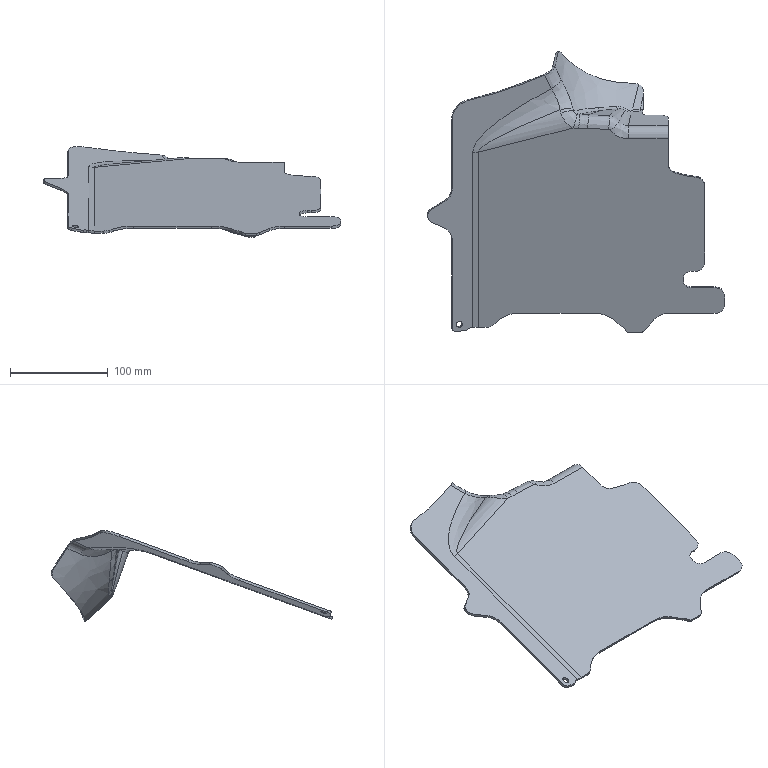Part | STEP file | K8D2-17C931-A-INS-01_id54_x_t | 1 solid | 123 faces | box 305 x 288.457 x 93.298 mm | volume 168343 mm3 | spline 83 | cylinder 26 | plane 14 | commonest cylinder face diameters 20 x6 8 x3 60 x3 17 x2 55 x2 200 x2